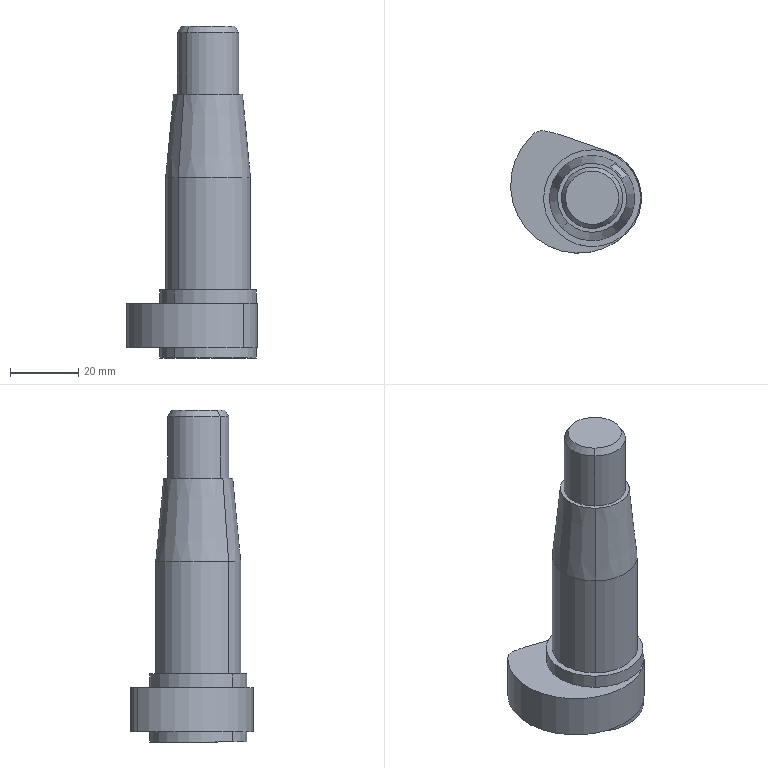Part | SolidWorks | features BaseBody 1 | 1 solid | 41 faces | box 38.423 x 35.937 x 97.5 mm | volume 48159 mm3 | plane 20 | cylinder 17 | cone 4 | commonest cylinder face diameters 28.5 x4 18 x2 25 x2 29 x2 6 x1 9 x1
STEP:
#1=CARTESIAN_POINT('',(-35.401,-41.494,71.636));
#2=VERTEX_POINT('',#1);
#3=CARTESIAN_POINT('',(-35.401,-41.494,85.05));
#4=VERTEX_POINT('',#3);
#5=CARTESIAN_POINT('',(-35.401,-41.494,99.25));
#6=DIRECTION('',(0.,0.,1.));
#7=VECTOR('',#6,1000.);
#8=LINE('',#5,#7);
#9=EDGE_CURVE('',#2,#4,#8,.T.);
#10=ORIENTED_EDGE('',*,*,#9,.F.);
#11=CARTESIAN_POINT('',(-32.752,-45.734,71.636));
#12=VERTEX_POINT('',#11);
#13=CARTESIAN_POINT('',(-44.463,-50.104,71.636));
#14=DIRECTION('',(0.,0.,-1.));
#15=DIRECTION('',(0.7009,0.7133,0.));
#16=AXIS2_PLACEMENT_3D('',#13,#14,#15);
#17=CIRCLE('',#16,12.5);
#18=EDGE_CURVE('',#2,#12,#17,.T.);
#19=ORIENTED_EDGE('',*,*,#18,.T.);
#20=CARTESIAN_POINT('',(-32.752,-45.734,85.05));
#21=VERTEX_POINT('',#20);
#22=CARTESIAN_POINT('',(-32.752,-45.734,99.25));
#23=DIRECTION('',(0.,0.,1.));
#24=VECTOR('',#23,1000.);
#25=LINE('',#22,#24);
#26=EDGE_CURVE('',#12,#21,#25,.T.);
#27=ORIENTED_EDGE('',*,*,#26,.T.);
#28=CARTESIAN_POINT('',(-44.463,-50.104,85.05));
#29=DIRECTION('',(0.,0.,1.));
#30=DIRECTION('',(-0.7009,-0.7133,0.));
#31=AXIS2_PLACEMENT_3D('',#28,#29,#30);
#32=CIRCLE('',#31,12.5);
#33=EDGE_CURVE('',#21,#4,#32,.T.);
#34=ORIENTED_EDGE('',*,*,#33,.T.);
#35=EDGE_LOOP('',(#10,#19,#27,#34));
#36=FACE_BOUND('',#35,.T.);
#37=CARTESIAN_POINT('',(-53.224,-59.019,99.25));
#38=VERTEX_POINT('',#37);
#39=CARTESIAN_POINT('',(-35.702,-41.188,99.25));
#40=VERTEX_POINT('',#39);
#41=CARTESIAN_POINT('',(-44.463,-50.104,99.25));
#42=DIRECTION('',(0.,0.,1.));
#43=DIRECTION('',(-0.7009,-0.7133,0.));
#44=AXIS2_PLACEMENT_3D('',#41,#42,#43);
#45=CIRCLE('',#44,12.5);
#46=EDGE_CURVE('',#38,#40,#45,.T.);
#47=ORIENTED_EDGE('',*,*,#46,.F.);
#48=CARTESIAN_POINT('',(-53.224,-59.019,66.25));
#49=VERTEX_POINT('',#48);
#50=CARTESIAN_POINT('',(-53.224,-59.019,99.25));
#51=DIRECTION('',(0.,0.,-1.));
#52=VECTOR('',#51,1000.);
#53=LINE('',#50,#52);
#54=EDGE_CURVE('',#38,#49,#53,.T.);
#55=ORIENTED_EDGE('',*,*,#54,.T.);
#56=CARTESIAN_POINT('',(-35.702,-41.188,66.25));
#57=VERTEX_POINT('',#56);
#58=CARTESIAN_POINT('',(-44.463,-50.104,66.25));
#59=DIRECTION('',(0.,0.,-1.));
#60=DIRECTION('',(0.7009,0.7133,0.));
#61=AXIS2_PLACEMENT_3D('',#58,#59,#60);
#62=CIRCLE('',#61,12.5);
#63=EDGE_CURVE('',#57,#49,#62,.T.);
#64=ORIENTED_EDGE('',*,*,#63,.F.);
#65=CARTESIAN_POINT('',(-35.702,-41.188,99.25));
#66=DIRECTION('',(0.,0.,-1.));
#67=VECTOR('',#66,1000.);
#68=LINE('',#65,#67);
#69=EDGE_CURVE('',#40,#57,#68,.T.);
#70=ORIENTED_EDGE('',*,*,#69,.F.);
#71=EDGE_LOOP('',(#47,#55,#64,#70));
#72=FACE_OUTER_BOUND('',#71,.T.);
#73=CARTESIAN_POINT('',(-44.463,-50.104,99.25));
#74=DIRECTION('',(0.,0.,-1.));
#75=DIRECTION('',(0.7009,0.7133,0.));
#76=AXIS2_PLACEMENT_3D('',#73,#74,#75);
#77=CYLINDRICAL_SURFACE('',#76,12.5);
#78=ADVANCED_FACE('',(#36,#72),#77,.T.);
#79=CARTESIAN_POINT('',(-34.3,-39.762,62.25));
#80=VERTEX_POINT('',#79);
#81=CARTESIAN_POINT('',(-39.674,-36.417,62.25));
#82=VERTEX_POINT('',#81);
#83=CARTESIAN_POINT('',(-44.463,-50.104,62.25));
#84=DIRECTION('',(0.,0.,1.));
#85=DIRECTION('',(-0.7009,-0.7133,0.));
#86=AXIS2_PLACEMENT_3D('',#83,#84,#85);
#87=CIRCLE('',#86,14.5);
#88=EDGE_CURVE('',#80,#82,#87,.T.);
#89=ORIENTED_EDGE('',*,*,#88,.F.);
#90=CARTESIAN_POINT('',(-34.3,-39.762,49.25));
#91=VERTEX_POINT('',#90);
#92=CARTESIAN_POINT('',(-34.3,-39.762,62.25));
#93=DIRECTION('',(0.,0.,-1.));
#94=VECTOR('',#93,1000.);
#95=LINE('',#92,#94);
#96=EDGE_CURVE('',#80,#91,#95,.T.);
#97=ORIENTED_EDGE('',*,*,#96,.T.);
#98=CARTESIAN_POINT('',(-39.674,-36.417,49.25));
#99=VERTEX_POINT('',#98);
#100=CARTESIAN_POINT('',(-44.463,-50.104,49.25));
#101=DIRECTION('',(0.,0.,1.));
#102=DIRECTION('',(-0.7009,-0.7133,0.));
#103=AXIS2_PLACEMENT_3D('',#100,#101,#102);
#104=CIRCLE('',#103,14.5);
#105=EDGE_CURVE('',#91,#99,#104,.T.);
#106=ORIENTED_EDGE('',*,*,#105,.T.);
#107=CARTESIAN_POINT('',(-39.674,-36.417,62.25));
#108=DIRECTION('',(0.,0.,-1.));
#109=VECTOR('',#108,1000.);
#110=LINE('',#107,#109);
#111=EDGE_CURVE('',#82,#99,#110,.T.);
#112=ORIENTED_EDGE('',*,*,#111,.F.);
#113=EDGE_LOOP('',(#89,#97,#106,#112));
#114=FACE_OUTER_BOUND('',#113,.T.);
#115=CARTESIAN_POINT('',(-44.463,-50.104,62.25));
#116=DIRECTION('',(0.,0.,-1.));
#117=DIRECTION('',(0.7009,0.7133,0.));
#118=AXIS2_PLACEMENT_3D('',#115,#116,#117);
#119=CYLINDRICAL_SURFACE('',#118,14.5);
#120=ADVANCED_FACE('',(#114),#119,.T.);
#121=CARTESIAN_POINT('',(-54.451,-60.268,46.25));
#122=VERTEX_POINT('',#121);
#123=CARTESIAN_POINT('',(-36.413,-38.345,46.25));
#124=VERTEX_POINT('',#123);
#125=CARTESIAN_POINT('',(-44.463,-50.104,46.25));
#126=DIRECTION('',(0.,0.,-1.));
#127=DIRECTION('',(0.7009,0.7133,0.));
#128=AXIS2_PLACEMENT_3D('',#125,#126,#127);
#129=CIRCLE('',#128,14.25);
#130=EDGE_CURVE('',#122,#124,#129,.T.);
#131=ORIENTED_EDGE('',*,*,#130,.F.);
#132=CARTESIAN_POINT('',(-54.451,-60.268,49.25));
#133=VERTEX_POINT('',#132);
#134=CARTESIAN_POINT('',(-54.451,-60.268,46.25));
#135=DIRECTION('',(0.,0.,1.));
#136=VECTOR('',#135,1000.);
#137=LINE('',#134,#136);
#138=EDGE_CURVE('',#122,#133,#137,.T.);
#139=ORIENTED_EDGE('',*,*,#138,.T.);
#140=CARTESIAN_POINT('',(-36.413,-38.345,49.25));
#141=VERTEX_POINT('',#140);
#142=CARTESIAN_POINT('',(-44.463,-50.104,49.25));
#143=DIRECTION('',(0.,0.,1.));
#144=DIRECTION('',(-0.7009,-0.7133,0.));
#145=AXIS2_PLACEMENT_3D('',#142,#143,#144);
#146=CIRCLE('',#145,14.25);
#147=EDGE_CURVE('',#141,#133,#146,.T.);
#148=ORIENTED_EDGE('',*,*,#147,.F.);
#149=CARTESIAN_POINT('',(-36.413,-38.345,46.25));
#150=DIRECTION('',(0.,0.,1.));
#151=VECTOR('',#150,1000.);
#152=LINE('',#149,#151);
#153=EDGE_CURVE('',#124,#141,#152,.T.);
#154=ORIENTED_EDGE('',*,*,#153,.F.);
#155=EDGE_LOOP('',(#131,#139,#148,#154));
#156=FACE_OUTER_BOUND('',#155,.T.);
#157=CARTESIAN_POINT('',(-44.463,-50.104,46.25));
#158=DIRECTION('',(0.,0.,1.));
#159=DIRECTION('',(-0.7009,-0.7133,0.));
#160=AXIS2_PLACEMENT_3D('',#157,#158,#159);
#161=CYLINDRICAL_SURFACE('',#160,14.25);
#162=ADVANCED_FACE('',(#156),#161,.T.);
#163=CARTESIAN_POINT('',(-51.571,-57.337,123.75));
#164=VERTEX_POINT('',#163);
#165=CARTESIAN_POINT('',(-37.355,-42.871,123.75));
#166=VERTEX_POINT('',#165);
#167=CARTESIAN_POINT('',(-44.463,-50.104,123.75));
#168=DIRECTION('',(0.,0.,-1.));
#169=DIRECTION('',(0.7009,0.7133,0.));
#170=AXIS2_PLACEMENT_3D('',#167,#168,#169);
#171=CIRCLE('',#170,10.141);
#172=EDGE_CURVE('',#164,#166,#171,.T.);
#173=ORIENTED_EDGE('',*,*,#172,.T.);
#174=CARTESIAN_POINT('',(-37.071,-42.582,119.547));
#175=VERTEX_POINT('',#174);
#176=CARTESIAN_POINT('',(-35.702,-41.188,99.25));
#177=DIRECTION('',(0.06718,0.06836,-0.9954));
#178=VECTOR('',#177,1000.);
#179=LINE('',#176,#178);
#180=EDGE_CURVE('',#166,#175,#179,.T.);
#181=ORIENTED_EDGE('',*,*,#180,.T.);
#182=CARTESIAN_POINT('',(-39.052,-41.03,119.351));
#183=VERTEX_POINT('',#182);
#184=CARTESIAN_POINT('',(-37.071,-42.582,119.547));
#185=CARTESIAN_POINT('',(-37.371,-42.288,119.547));
#186=CARTESIAN_POINT('',(-37.69,-42.007,119.531));
#187=CARTESIAN_POINT('',(-38.352,-41.489,119.467));
#188=CARTESIAN_POINT('',(-38.696,-41.25,119.418));
#189=CARTESIAN_POINT('',(-39.052,-41.03,119.351));
#190=B_SPLINE_CURVE_WITH_KNOTS('',3,(#184,#185,#186,#187,#188,#189),.UNSPECIFIED.,.F.,.F.,(4,2,4),(0.002522,0.003775,0.005027),.UNSPECIFIED.);
#191=EDGE_CURVE('',#175,#183,#190,.T.);
#192=ORIENTED_EDGE('',*,*,#191,.T.);
#193=CARTESIAN_POINT('',(-37.921,-39.88,103.01));
#194=VERTEX_POINT('',#193);
#195=CARTESIAN_POINT('',(-37.921,-39.88,103.01));
#196=CARTESIAN_POINT('',(-37.971,-39.931,103.745));
#197=CARTESIAN_POINT('',(-38.022,-39.983,104.479));
#198=CARTESIAN_POINT('',(-38.398,-40.365,109.927));
#199=CARTESIAN_POINT('',(-38.724,-40.697,114.639));
#200=CARTESIAN_POINT('',(-39.052,-41.03,119.351));
#201=B_SPLINE_CURVE_WITH_KNOTS('',3,(#195,#196,#197,#198,#199,#200),.UNSPECIFIED.,.F.,.F.,(4,2,4),(0.,0.1349,1.),.UNSPECIFIED.);
#202=EDGE_CURVE('',#194,#183,#201,.T.);
#203=ORIENTED_EDGE('',*,*,#202,.F.);
#204=CARTESIAN_POINT('',(-35.947,-41.438,102.891));
#205=VERTEX_POINT('',#204);
#206=CARTESIAN_POINT('',(-37.921,-39.88,103.01));
#207=CARTESIAN_POINT('',(-37.204,-40.329,102.926));
#208=CARTESIAN_POINT('',(-36.546,-40.849,102.891));
#209=CARTESIAN_POINT('',(-35.947,-41.438,102.891));
#210=B_SPLINE_CURVE_WITH_KNOTS('',3,(#206,#207,#208,#209),.UNSPECIFIED.,.F.,.F.,(4,4),(0.,0.002514),.UNSPECIFIED.);
#211=EDGE_CURVE('',#194,#205,#210,.T.);
#212=ORIENTED_EDGE('',*,*,#211,.T.);
#213=CARTESIAN_POINT('',(-35.702,-41.188,99.25));
#214=DIRECTION('',(0.06718,0.06836,-0.9954));
#215=VECTOR('',#214,1000.);
#216=LINE('',#213,#215);
#217=EDGE_CURVE('',#205,#40,#216,.T.);
#218=ORIENTED_EDGE('',*,*,#217,.T.);
#219=CARTESIAN_POINT('',(-44.463,-50.104,99.25));
#220=DIRECTION('',(0.,0.,1.));
#221=DIRECTION('',(-0.7009,-0.7133,0.));
#222=AXIS2_PLACEMENT_3D('',#219,#220,#221);
#223=CIRCLE('',#222,12.5);
#224=EDGE_CURVE('',#40,#38,#223,.T.);
#225=ORIENTED_EDGE('',*,*,#224,.T.);
#226=CARTESIAN_POINT('',(-53.224,-59.019,99.25));
#227=DIRECTION('',(-0.06718,-0.06836,-0.9954));
#228=VECTOR('',#227,1000.);
#229=LINE('',#226,#228);
#230=EDGE_CURVE('',#164,#38,#229,.T.);
#231=ORIENTED_EDGE('',*,*,#230,.F.);
#232=EDGE_LOOP('',(#173,#181,#192,#203,#212,#218,#225,#231));
#233=FACE_OUTER_BOUND('',#232,.T.);
#234=CARTESIAN_POINT('',(-44.463,-50.104,99.25));
#235=DIRECTION('',(0.,0.,-1.));
#236=DIRECTION('',(-0.7009,-0.7133,0.));
#237=AXIS2_PLACEMENT_3D('',#234,#235,#236);
#238=CONICAL_SURFACE('',#237,12.5,0.09599);
#239=ADVANCED_FACE('',(#233),#238,.T.);
#240=CARTESIAN_POINT('',(-38.155,-43.685,141.75));
#241=VERTEX_POINT('',#240);
#242=CARTESIAN_POINT('',(-50.771,-56.523,141.75));
#243=VERTEX_POINT('',#242);
#244=CARTESIAN_POINT('',(-44.463,-50.104,141.75));
#245=DIRECTION('',(0.,0.,-1.));
#246=DIRECTION('',(0.7009,0.7133,0.));
#247=AXIS2_PLACEMENT_3D('',#244,#245,#246);
#248=CIRCLE('',#247,9.);
#249=EDGE_CURVE('',#241,#243,#248,.T.);
#250=ORIENTED_EDGE('',*,*,#249,.T.);
#251=CARTESIAN_POINT('',(-50.771,-56.523,123.75));
#252=VERTEX_POINT('',#251);
#253=CARTESIAN_POINT('',(-50.771,-56.523,169.206));
#254=DIRECTION('',(0.,0.,-1.));
#255=VECTOR('',#254,1000.);
#256=LINE('',#253,#255);
#257=EDGE_CURVE('',#243,#252,#256,.T.);
#258=ORIENTED_EDGE('',*,*,#257,.T.);
#259=CARTESIAN_POINT('',(-38.155,-43.685,123.75));
#260=VERTEX_POINT('',#259);
#261=CARTESIAN_POINT('',(-44.463,-50.104,123.75));
#262=DIRECTION('',(0.,0.,1.));
#263=DIRECTION('',(0.7009,0.7133,0.));
#264=AXIS2_PLACEMENT_3D('',#261,#262,#263);
#265=CIRCLE('',#264,9.);
#266=EDGE_CURVE('',#252,#260,#265,.T.);
#267=ORIENTED_EDGE('',*,*,#266,.T.);
#268=CARTESIAN_POINT('',(-38.155,-43.685,169.206));
#269=DIRECTION('',(0.,0.,-1.));
#270=VECTOR('',#269,1000.);
#271=LINE('',#268,#270);
#272=EDGE_CURVE('',#241,#260,#271,.T.);
#273=ORIENTED_EDGE('',*,*,#272,.F.);
#274=EDGE_LOOP('',(#250,#258,#267,#273));
#275=FACE_OUTER_BOUND('',#274,.T.);
#276=CARTESIAN_POINT('',(-44.463,-50.104,169.206));
#277=DIRECTION('',(0.,0.,-1.));
#278=DIRECTION('',(0.7009,0.7133,0.));
#279=AXIS2_PLACEMENT_3D('',#276,#277,#278);
#280=CYLINDRICAL_SURFACE('',#279,9.);
#281=ADVANCED_FACE('',(#275),#280,.T.);
#282=CARTESIAN_POINT('',(-54.451,-60.268,62.25));
#283=VERTEX_POINT('',#282);
#284=CARTESIAN_POINT('',(-34.475,-39.94,62.25));
#285=VERTEX_POINT('',#284);
#286=CARTESIAN_POINT('',(-44.463,-50.104,62.25));
#287=DIRECTION('',(0.,0.,1.));
#288=DIRECTION('',(-0.7009,-0.7133,0.));
#289=AXIS2_PLACEMENT_3D('',#286,#287,#288);
#290=CIRCLE('',#289,14.25);
#291=EDGE_CURVE('',#283,#285,#290,.T.);
#292=ORIENTED_EDGE('',*,*,#291,.T.);
#293=CARTESIAN_POINT('',(-34.475,-39.94,66.25));
#294=VERTEX_POINT('',#293);
#295=CARTESIAN_POINT('',(-34.475,-39.94,46.25));
#296=DIRECTION('',(0.,0.,1.));
#297=VECTOR('',#296,1000.);
#298=LINE('',#295,#297);
#299=EDGE_CURVE('',#285,#294,#298,.T.);
#300=ORIENTED_EDGE('',*,*,#299,.T.);
#301=CARTESIAN_POINT('',(-54.451,-60.268,66.25));
#302=VERTEX_POINT('',#301);
#303=CARTESIAN_POINT('',(-44.463,-50.104,66.25));
#304=DIRECTION('',(0.,0.,-1.));
#305=DIRECTION('',(0.7009,0.7133,0.));
#306=AXIS2_PLACEMENT_3D('',#303,#304,#305);
#307=CIRCLE('',#306,14.25);
#308=EDGE_CURVE('',#294,#302,#307,.T.);
#309=ORIENTED_EDGE('',*,*,#308,.T.);
#310=CARTESIAN_POINT('',(-54.451,-60.268,46.25));
#311=DIRECTION('',(0.,0.,1.));
#312=VECTOR('',#311,1000.);
#313=LINE('',#310,#312);
#314=EDGE_CURVE('',#283,#302,#313,.T.);
#315=ORIENTED_EDGE('',*,*,#314,.F.);
#316=EDGE_LOOP('',(#292,#300,#309,#315));
#317=FACE_OUTER_BOUND('',#316,.T.);
#318=CARTESIAN_POINT('',(-44.463,-50.104,46.25));
#319=DIRECTION('',(0.,0.,1.));
#320=DIRECTION('',(-0.7009,-0.7133,0.));
#321=AXIS2_PLACEMENT_3D('',#318,#319,#320);
#322=CYLINDRICAL_SURFACE('',#321,14.25);
#323=ADVANCED_FACE('',(#317),#322,.T.);
#324=CARTESIAN_POINT('',(-49.962,-55.699,143.75));
#325=VERTEX_POINT('',#324);
#326=CARTESIAN_POINT('',(-38.964,-44.508,143.75));
#327=VERTEX_POINT('',#326);
#328=CARTESIAN_POINT('',(-44.463,-50.104,143.75));
#329=DIRECTION('',(0.,0.,1.));
#330=DIRECTION('',(0.7009,0.7133,0.));
#331=AXIS2_PLACEMENT_3D('',#328,#329,#330);
#332=CIRCLE('',#331,7.845);
#333=EDGE_CURVE('',#325,#327,#332,.T.);
#334=ORIENTED_EDGE('',*,*,#333,.F.);
#335=CARTESIAN_POINT('',(-50.771,-56.523,141.75));
#336=DIRECTION('',(-0.3505,-0.3566,-0.866));
#337=VECTOR('',#336,1000.);
#338=LINE('',#335,#337);
#339=EDGE_CURVE('',#325,#243,#338,.T.);
#340=ORIENTED_EDGE('',*,*,#339,.T.);
#341=ORIENTED_EDGE('',*,*,#249,.F.);
#342=CARTESIAN_POINT('',(-38.155,-43.685,141.75));
#343=DIRECTION('',(0.3505,0.3566,-0.866));
#344=VECTOR('',#343,1000.);
#345=LINE('',#342,#344);
#346=EDGE_CURVE('',#327,#241,#345,.T.);
#347=ORIENTED_EDGE('',*,*,#346,.F.);
#348=EDGE_LOOP('',(#334,#340,#341,#347));
#349=FACE_OUTER_BOUND('',#348,.T.);
#350=CARTESIAN_POINT('',(-44.463,-50.104,141.75));
#351=DIRECTION('',(0.,0.,-1.));
#352=DIRECTION('',(0.7009,0.7133,0.));
#353=AXIS2_PLACEMENT_3D('',#350,#351,#352);
#354=CONICAL_SURFACE('',#353,9.,0.5236);
#355=ADVANCED_FACE('',(#349),#354,.T.);
#356=CARTESIAN_POINT('',(-38.181,-49.126,85.05));
#357=VERTEX_POINT('',#356);
#358=CARTESIAN_POINT('',(-38.181,-49.126,71.636));
#359=VERTEX_POINT('',#358);
#360=CARTESIAN_POINT('',(-38.181,-49.126,85.05));
#361=DIRECTION('',(0.,0.,-1.));
#362=VECTOR('',#361,1000.);
#363=LINE('',#360,#362);
#364=EDGE_CURVE('',#357,#359,#363,.T.);
#365=ORIENTED_EDGE('',*,*,#364,.T.);
#366=CARTESIAN_POINT('',(-40.83,-44.886,71.636));
#367=VERTEX_POINT('',#366);
#368=CARTESIAN_POINT('',(-40.83,-44.886,71.636));
#369=DIRECTION('',(0.5299,-0.848,0.));
#370=VECTOR('',#369,1000.);
#371=LINE('',#368,#370);
#372=EDGE_CURVE('',#367,#359,#371,.T.);
#373=ORIENTED_EDGE('',*,*,#372,.F.);
#374=CARTESIAN_POINT('',(-40.83,-44.886,85.05));
#375=VERTEX_POINT('',#374);
#376=CARTESIAN_POINT('',(-40.83,-44.886,85.05));
#377=DIRECTION('',(0.,0.,-1.));
#378=VECTOR('',#377,1000.);
#379=LINE('',#376,#378);
#380=EDGE_CURVE('',#375,#367,#379,.T.);
#381=ORIENTED_EDGE('',*,*,#380,.F.);
#382=CARTESIAN_POINT('',(-40.83,-44.886,85.05));
#383=DIRECTION('',(0.5299,-0.848,0.));
#384=VECTOR('',#383,1000.);
#385=LINE('',#382,#384);
#386=EDGE_CURVE('',#375,#357,#385,.T.);
#387=ORIENTED_EDGE('',*,*,#386,.T.);
#388=EDGE_LOOP('',(#365,#373,#381,#387));
#389=FACE_OUTER_BOUND('',#388,.T.);
#390=CARTESIAN_POINT('',(-40.83,-44.886,85.05));
#391=DIRECTION('',(-0.848,-0.5299,0.));
#392=DIRECTION('',(-0.5299,0.848,0.));
#393=AXIS2_PLACEMENT_3D('',#390,#391,#392);
#394=PLANE('',#393);
#395=ADVANCED_FACE('',(#389),#394,.F.);
#396=CARTESIAN_POINT('',(-38.181,-49.126,71.636));
#397=DIRECTION('',(0.848,0.5299,0.));
#398=VECTOR('',#397,1000.);
#399=LINE('',#396,#398);
#400=EDGE_CURVE('',#359,#12,#399,.T.);
#401=ORIENTED_EDGE('',*,*,#400,.F.);
#402=ORIENTED_EDGE('',*,*,#364,.F.);
#403=CARTESIAN_POINT('',(-38.181,-49.126,85.05));
#404=DIRECTION('',(-0.848,-0.5299,0.));
#405=VECTOR('',#404,1000.);
#406=LINE('',#403,#405);
#407=EDGE_CURVE('',#21,#357,#406,.T.);
#408=ORIENTED_EDGE('',*,*,#407,.F.);
#409=ORIENTED_EDGE('',*,*,#26,.F.);
#410=EDGE_LOOP('',(#401,#402,#408,#409));
#411=FACE_OUTER_BOUND('',#410,.T.);
#412=CARTESIAN_POINT('',(-38.181,-49.126,71.636));
#413=DIRECTION('',(0.5299,-0.848,0.));
#414=DIRECTION('',(0.,0.,-1.));
#415=AXIS2_PLACEMENT_3D('',#412,#413,#414);
#416=PLANE('',#415);
#417=ADVANCED_FACE('',(#411),#416,.F.);
#418=ORIENTED_EDGE('',*,*,#9,.T.);
#419=CARTESIAN_POINT('',(-40.83,-44.886,85.05));
#420=DIRECTION('',(-0.848,-0.5299,0.));
#421=VECTOR('',#420,1000.);
#422=LINE('',#419,#421);
#423=EDGE_CURVE('',#4,#375,#422,.T.);
#424=ORIENTED_EDGE('',*,*,#423,.T.);
#425=ORIENTED_EDGE('',*,*,#380,.T.);
#426=CARTESIAN_POINT('',(-40.83,-44.886,71.636));
#427=DIRECTION('',(0.848,0.5299,0.));
#428=VECTOR('',#427,1000.);
#429=LINE('',#426,#428);
#430=EDGE_CURVE('',#367,#2,#429,.T.);
#431=ORIENTED_EDGE('',*,*,#430,.T.);
#432=EDGE_LOOP('',(#418,#424,#425,#431));
#433=FACE_OUTER_BOUND('',#432,.T.);
#434=CARTESIAN_POINT('',(-40.83,-44.886,71.636));
#435=DIRECTION('',(0.5299,-0.848,0.));
#436=DIRECTION('',(0.,0.,-1.));
#437=AXIS2_PLACEMENT_3D('',#434,#435,#436);
#438=PLANE('',#437);
#439=ADVANCED_FACE('',(#433),#438,.T.);
#440=ORIENTED_EDGE('',*,*,#430,.F.);
#441=ORIENTED_EDGE('',*,*,#372,.T.);
#442=ORIENTED_EDGE('',*,*,#400,.T.);
#443=ORIENTED_EDGE('',*,*,#18,.F.);
#444=EDGE_LOOP('',(#440,#441,#442,#443));
#445=FACE_OUTER_BOUND('',#444,.T.);
#446=CARTESIAN_POINT('',(-40.83,-44.886,71.636));
#447=DIRECTION('',(0.,0.,-1.));
#448=DIRECTION('',(0.,-1.,0.));
#449=AXIS2_PLACEMENT_3D('',#446,#447,#448);
#450=PLANE('',#449);
#451=ADVANCED_FACE('',(#445),#450,.F.);
#452=ORIENTED_EDGE('',*,*,#407,.T.);
#453=ORIENTED_EDGE('',*,*,#386,.F.);
#454=ORIENTED_EDGE('',*,*,#423,.F.);
#455=ORIENTED_EDGE('',*,*,#33,.F.);
#456=EDGE_LOOP('',(#452,#453,#454,#455));
#457=FACE_OUTER_BOUND('',#456,.T.);
#458=CARTESIAN_POINT('',(-40.83,-44.886,85.05));
#459=DIRECTION('',(0.,0.,1.));
#460=DIRECTION('',(0.,-1.,0.));
#461=AXIS2_PLACEMENT_3D('',#458,#459,#460);
#462=PLANE('',#461);
#463=ADVANCED_FACE('',(#457),#462,.F.);
#464=CARTESIAN_POINT('',(-31.241,-44.79,46.25));
#465=VERTEX_POINT('',#464);
#466=CARTESIAN_POINT('',(-35.995,-47.76,46.25));
#467=VERTEX_POINT('',#466);
#468=CARTESIAN_POINT('',(-43.138,-52.224,46.25));
#469=DIRECTION('',(-0.848,-0.5299,0.));
#470=VECTOR('',#469,1000.);
#471=LINE('',#468,#470);
#472=EDGE_CURVE('',#465,#467,#471,.T.);
#473=ORIENTED_EDGE('',*,*,#472,.T.);
#474=CARTESIAN_POINT('',(-35.995,-47.76,53.733));
#475=VERTEX_POINT('',#474);
#476=CARTESIAN_POINT('',(-35.995,-47.76,53.733));
#477=DIRECTION('',(0.,0.,-1.));
#478=VECTOR('',#477,1000.);
#479=LINE('',#476,#478);
#480=EDGE_CURVE('',#475,#467,#479,.T.);
#481=ORIENTED_EDGE('',*,*,#480,.F.);
#482=CARTESIAN_POINT('',(-31.026,-44.655,53.733));
#483=VERTEX_POINT('',#482);
#484=CARTESIAN_POINT('',(-35.995,-47.76,53.733));
#485=DIRECTION('',(-0.848,-0.5299,0.));
#486=VECTOR('',#485,1000.);
#487=LINE('',#484,#486);
#488=EDGE_CURVE('',#483,#475,#487,.T.);
#489=ORIENTED_EDGE('',*,*,#488,.F.);
#490=CARTESIAN_POINT('',(-31.026,-44.655,49.25));
#491=VERTEX_POINT('',#490);
#492=CARTESIAN_POINT('',(-31.026,-44.655,62.25));
#493=DIRECTION('',(0.,0.,1.));
#494=VECTOR('',#493,1000.);
#495=LINE('',#492,#494);
#496=EDGE_CURVE('',#491,#483,#495,.T.);
#497=ORIENTED_EDGE('',*,*,#496,.F.);
#498=CARTESIAN_POINT('',(-31.241,-44.79,49.25));
#499=VERTEX_POINT('',#498);
#500=CARTESIAN_POINT('',(-43.138,-52.224,49.25));
#501=DIRECTION('',(0.848,0.5299,0.));
#502=VECTOR('',#501,1000.);
#503=LINE('',#500,#502);
#504=EDGE_CURVE('',#499,#491,#503,.T.);
#505=ORIENTED_EDGE('',*,*,#504,.F.);
#506=CARTESIAN_POINT('',(-31.241,-44.79,46.25));
#507=DIRECTION('',(0.,0.,1.));
#508=VECTOR('',#507,1000.);
#509=LINE('',#506,#508);
#510=EDGE_CURVE('',#465,#499,#509,.T.);
#511=ORIENTED_EDGE('',*,*,#510,.F.);
#512=EDGE_LOOP('',(#473,#481,#489,#497,#505,#511));
#513=FACE_OUTER_BOUND('',#512,.T.);
#514=CARTESIAN_POINT('',(-35.995,-47.76,40.466));
#515=DIRECTION('',(0.5299,-0.848,0.));
#516=DIRECTION('',(0.,0.,-1.));
#517=AXIS2_PLACEMENT_3D('',#514,#515,#516);
#518=PLANE('',#517);
#519=ADVANCED_FACE('',(#513),#518,.F.);
#520=CARTESIAN_POINT('',(-38.644,-43.52,46.25));
#521=VERTEX_POINT('',#520);
#522=CARTESIAN_POINT('',(-37.32,-45.64,46.25));
#523=DIRECTION('',(-0.5299,0.848,0.));
#524=VECTOR('',#523,1000.);
#525=LINE('',#522,#524);
#526=EDGE_CURVE('',#467,#521,#525,.T.);
#527=ORIENTED_EDGE('',*,*,#526,.T.);
#528=CARTESIAN_POINT('',(-38.644,-43.52,53.733));
#529=VERTEX_POINT('',#528);
#530=CARTESIAN_POINT('',(-38.644,-43.52,53.733));
#531=DIRECTION('',(0.,0.,-1.));
#532=VECTOR('',#531,1000.);
#533=LINE('',#530,#532);
#534=EDGE_CURVE('',#529,#521,#533,.T.);
#535=ORIENTED_EDGE('',*,*,#534,.F.);
#536=CARTESIAN_POINT('',(-38.644,-43.52,53.733));
#537=DIRECTION('',(0.5299,-0.848,0.));
#538=VECTOR('',#537,1000.);
#539=LINE('',#536,#538);
#540=EDGE_CURVE('',#529,#475,#539,.T.);
#541=ORIENTED_EDGE('',*,*,#540,.T.);
#542=ORIENTED_EDGE('',*,*,#480,.T.);
#543=EDGE_LOOP('',(#527,#535,#541,#542));
#544=FACE_OUTER_BOUND('',#543,.T.);
#545=CARTESIAN_POINT('',(-38.644,-43.52,53.733));
#546=DIRECTION('',(-0.848,-0.5299,0.));
#547=DIRECTION('',(-0.5299,0.848,0.));
#548=AXIS2_PLACEMENT_3D('',#545,#546,#547);
#549=PLANE('',#548);
#550=ADVANCED_FACE('',(#544),#549,.F.);
#551=CARTESIAN_POINT('',(-33.675,-40.415,49.25));
#552=VERTEX_POINT('',#551);
#553=CARTESIAN_POINT('',(-33.675,-40.415,53.733));
#554=VERTEX_POINT('',#553);
#555=CARTESIAN_POINT('',(-33.675,-40.415,62.25));
#556=DIRECTION('',(0.,0.,1.));
#557=VECTOR('',#556,1000.);
#558=LINE('',#555,#557);
#559=EDGE_CURVE('',#552,#554,#558,.T.);
#560=ORIENTED_EDGE('',*,*,#559,.T.);
#561=CARTESIAN_POINT('',(-38.644,-43.52,53.733));
#562=DIRECTION('',(-0.848,-0.5299,0.));
#563=VECTOR('',#562,1000.);
#564=LINE('',#561,#563);
#565=EDGE_CURVE('',#554,#529,#564,.T.);
#566=ORIENTED_EDGE('',*,*,#565,.T.);
#567=ORIENTED_EDGE('',*,*,#534,.T.);
#568=CARTESIAN_POINT('',(-38.258,-43.279,46.25));
#569=VERTEX_POINT('',#568);
#570=CARTESIAN_POINT('',(-45.788,-47.984,46.25));
#571=DIRECTION('',(-0.848,-0.5299,0.));
#572=VECTOR('',#571,1000.);
#573=LINE('',#570,#572);
#574=EDGE_CURVE('',#569,#521,#573,.T.);
#575=ORIENTED_EDGE('',*,*,#574,.F.);
#576=CARTESIAN_POINT('',(-38.258,-43.279,49.25));
#577=VERTEX_POINT('',#576);
#578=CARTESIAN_POINT('',(-38.258,-43.279,43.06));
#579=DIRECTION('',(0.,0.,1.));
#580=VECTOR('',#579,1000.);
#581=LINE('',#578,#580);
#582=EDGE_CURVE('',#569,#577,#581,.T.);
#583=ORIENTED_EDGE('',*,*,#582,.T.);
#584=CARTESIAN_POINT('',(-45.788,-47.984,49.25));
#585=DIRECTION('',(0.848,0.5299,0.));
#586=VECTOR('',#585,1000.);
#587=LINE('',#584,#586);
#588=EDGE_CURVE('',#577,#552,#587,.T.);
#589=ORIENTED_EDGE('',*,*,#588,.T.);
#590=EDGE_LOOP('',(#560,#566,#567,#575,#583,#589));
#591=FACE_OUTER_BOUND('',#590,.T.);
#592=CARTESIAN_POINT('',(-38.644,-43.52,40.466));
#593=DIRECTION('',(0.5299,-0.848,0.));
#594=DIRECTION('',(0.,0.,-1.));
#595=AXIS2_PLACEMENT_3D('',#592,#593,#594);
#596=PLANE('',#595);
#597=ADVANCED_FACE('',(#591),#596,.T.);
#598=ORIENTED_EDGE('',*,*,#488,.T.);
#599=ORIENTED_EDGE('',*,*,#540,.F.);
#600=ORIENTED_EDGE('',*,*,#565,.F.);
#601=CARTESIAN_POINT('',(-44.463,-50.104,53.733));
#602=DIRECTION('',(0.,0.,1.));
#603=DIRECTION('',(-0.7009,-0.7133,0.));
#604=AXIS2_PLACEMENT_3D('',#601,#602,#603);
#605=CIRCLE('',#604,14.5);
#606=EDGE_CURVE('',#483,#554,#605,.T.);
#607=ORIENTED_EDGE('',*,*,#606,.F.);
#608=EDGE_LOOP('',(#598,#599,#600,#607));
#609=FACE_OUTER_BOUND('',#608,.T.);
#610=CARTESIAN_POINT('',(-38.644,-43.52,53.733));
#611=DIRECTION('',(0.,0.,1.));
#612=DIRECTION('',(0.,-1.,0.));
#613=AXIS2_PLACEMENT_3D('',#610,#611,#612);
#614=PLANE('',#613);
#615=ADVANCED_FACE('',(#609),#614,.F.);
#616=ORIENTED_EDGE('',*,*,#153,.T.);
#617=CARTESIAN_POINT('',(-39.786,-41.778,49.25));
#618=VERTEX_POINT('',#617);
#619=CARTESIAN_POINT('',(-30.821,-32.655,49.25));
#620=DIRECTION('',(-0.7009,-0.7133,0.));
#621=VECTOR('',#620,1000.);
#622=LINE('',#619,#621);
#623=EDGE_CURVE('',#141,#618,#622,.T.);
#624=ORIENTED_EDGE('',*,*,#623,.T.);
#625=CARTESIAN_POINT('',(-39.786,-41.778,46.25));
#626=VERTEX_POINT('',#625);
#627=CARTESIAN_POINT('',(-39.786,-41.778,43.06));
#628=DIRECTION('',(0.,0.,-1.));
#629=VECTOR('',#628,1000.);
#630=LINE('',#627,#629);
#631=EDGE_CURVE('',#618,#626,#630,.T.);
#632=ORIENTED_EDGE('',*,*,#631,.T.);
#633=CARTESIAN_POINT('',(-46.246,-48.352,46.25));
#634=DIRECTION('',(-0.7009,-0.7133,0.));
#635=VECTOR('',#634,1000.);
#636=LINE('',#633,#635);
#637=EDGE_CURVE('',#124,#626,#636,.T.);
#638=ORIENTED_EDGE('',*,*,#637,.F.);
#639=EDGE_LOOP('',(#616,#624,#632,#638));
#640=FACE_OUTER_BOUND('',#639,.T.);
#641=CARTESIAN_POINT('',(-30.821,-32.655,49.25));
#642=DIRECTION('',(0.7133,-0.7009,0.));
#643=DIRECTION('',(0.,0.,-1.));
#644=AXIS2_PLACEMENT_3D('',#641,#642,#643);
#645=PLANE('',#644);
#646=ADVANCED_FACE('',(#640),#645,.T.);
#647=CARTESIAN_POINT('',(-35.485,-44.535,119.351));
#648=VERTEX_POINT('',#647);
#649=CARTESIAN_POINT('',(-34.355,-43.384,103.01));
#650=VERTEX_POINT('',#649);
#651=CARTESIAN_POINT('',(-31.587,-40.568,111.65));
#652=DIRECTION('',(0.7133,-0.7009,0.));
#653=DIRECTION('',(0.,0.,1.));
#654=AXIS2_PLACEMENT_3D('',#651,#652,#653);
#655=CIRCLE('',#654,9.5);
#656=EDGE_CURVE('',#648,#650,#655,.T.);
#657=ORIENTED_EDGE('',*,*,#656,.F.);
#658=CARTESIAN_POINT('',(-34.355,-43.384,103.01));
#659=CARTESIAN_POINT('',(-34.405,-43.436,103.745));
#660=CARTESIAN_POINT('',(-34.456,-43.487,104.479));
#661=CARTESIAN_POINT('',(-34.832,-43.87,109.927));
#662=CARTESIAN_POINT('',(-35.158,-44.202,114.639));
#663=CARTESIAN_POINT('',(-35.485,-44.535,119.351));
#664=B_SPLINE_CURVE_WITH_KNOTS('',3,(#658,#659,#660,#661,#662,#663),.UNSPECIFIED.,.F.,.F.,(4,2,4),(0.,0.1349,1.),.UNSPECIFIED.);
#665=EDGE_CURVE('',#650,#648,#664,.T.);
#666=ORIENTED_EDGE('',*,*,#665,.F.);
#667=EDGE_LOOP('',(#657,#666));
#668=FACE_OUTER_BOUND('',#667,.T.);
#669=CARTESIAN_POINT('',(-31.587,-40.568,111.65));
#670=DIRECTION('',(0.7133,-0.7009,0.));
#671=DIRECTION('',(0.,0.,-1.));
#672=AXIS2_PLACEMENT_3D('',#669,#670,#671);
#673=PLANE('',#672);
#674=ADVANCED_FACE('',(#668),#673,.F.);
#675=ORIENTED_EDGE('',*,*,#202,.T.);
#676=CARTESIAN_POINT('',(-35.153,-37.063,111.65));
#677=DIRECTION('',(0.7133,-0.7009,0.));
#678=DIRECTION('',(0.,0.,1.));
#679=AXIS2_PLACEMENT_3D('',#676,#677,#678);
#680=CIRCLE('',#679,9.5);
#681=EDGE_CURVE('',#183,#194,#680,.T.);
#682=ORIENTED_EDGE('',*,*,#681,.T.);
#683=EDGE_LOOP('',(#675,#682));
#684=FACE_OUTER_BOUND('',#683,.T.);
#685=CARTESIAN_POINT('',(-35.153,-37.063,111.65));
#686=DIRECTION('',(0.7133,-0.7009,0.));
#687=DIRECTION('',(0.,0.,-1.));
#688=AXIS2_PLACEMENT_3D('',#685,#686,#687);
#689=PLANE('',#688);
#690=ADVANCED_FACE('',(#684),#689,.T.);
#691=ORIENTED_EDGE('',*,*,#656,.T.);
#692=CARTESIAN_POINT('',(-35.947,-41.438,102.891));
#693=CARTESIAN_POINT('',(-35.65,-41.731,102.891));
#694=CARTESIAN_POINT('',(-35.366,-42.041,102.9));
#695=CARTESIAN_POINT('',(-34.832,-42.693,102.939));
#696=CARTESIAN_POINT('',(-34.584,-43.032,102.968));
#697=CARTESIAN_POINT('',(-34.355,-43.384,103.01));
#698=B_SPLINE_CURVE_WITH_KNOTS('',3,(#692,#693,#694,#695,#696,#697),.UNSPECIFIED.,.F.,.F.,(4,2,4),(0.002514,0.003763,0.005012),.UNSPECIFIED.);
#699=EDGE_CURVE('',#205,#650,#698,.T.);
#700=ORIENTED_EDGE('',*,*,#699,.F.);
#701=ORIENTED_EDGE('',*,*,#211,.F.);
#702=ORIENTED_EDGE('',*,*,#681,.F.);
#703=ORIENTED_EDGE('',*,*,#191,.F.);
#704=CARTESIAN_POINT('',(-35.485,-44.535,119.351));
#705=CARTESIAN_POINT('',(-35.94,-43.826,119.486));
#706=CARTESIAN_POINT('',(-36.468,-43.175,119.547));
#707=CARTESIAN_POINT('',(-37.071,-42.582,119.547));
#708=B_SPLINE_CURVE_WITH_KNOTS('',3,(#704,#705,#706,#707),.UNSPECIFIED.,.F.,.F.,(4,4),(0.,0.002522),.UNSPECIFIED.);
#709=EDGE_CURVE('',#648,#175,#708,.T.);
#710=ORIENTED_EDGE('',*,*,#709,.F.);
#711=EDGE_LOOP('',(#691,#700,#701,#702,#703,#710));
#712=FACE_OUTER_BOUND('',#711,.T.);
#713=CARTESIAN_POINT('',(-35.153,-37.063,111.65));
#714=DIRECTION('',(0.7133,-0.7009,0.));
#715=DIRECTION('',(0.,0.,1.));
#716=AXIS2_PLACEMENT_3D('',#713,#714,#715);
#717=CYLINDRICAL_SURFACE('',#716,9.5);
#718=ADVANCED_FACE('',(#712),#717,.F.);
#719=ORIENTED_EDGE('',*,*,#339,.F.);
#720=CARTESIAN_POINT('',(-44.463,-50.104,143.75));
#721=DIRECTION('',(0.,0.,1.));
#722=DIRECTION('',(0.7009,0.7133,0.));
#723=AXIS2_PLACEMENT_3D('',#720,#721,#722);
#724=CIRCLE('',#723,7.845);
#725=EDGE_CURVE('',#327,#325,#724,.T.);
#726=ORIENTED_EDGE('',*,*,#725,.F.);
#727=ORIENTED_EDGE('',*,*,#346,.T.);
#728=CARTESIAN_POINT('',(-44.463,-50.104,141.75));
#729=DIRECTION('',(0.,0.,-1.));
#730=DIRECTION('',(0.7009,0.7133,0.));
#731=AXIS2_PLACEMENT_3D('',#728,#729,#730);
#732=CIRCLE('',#731,9.);
#733=EDGE_CURVE('',#243,#241,#732,.T.);
#734=ORIENTED_EDGE('',*,*,#733,.F.);
#735=EDGE_LOOP('',(#719,#726,#727,#734));
#736=FACE_OUTER_BOUND('',#735,.T.);
#737=CARTESIAN_POINT('',(-44.463,-50.104,141.75));
#738=DIRECTION('',(0.,0.,-1.));
#739=DIRECTION('',(0.7009,0.7133,0.));
#740=AXIS2_PLACEMENT_3D('',#737,#738,#739);
#741=CONICAL_SURFACE('',#740,9.,0.5236);
#742=ADVANCED_FACE('',(#736),#741,.T.);
#743=CARTESIAN_POINT('',(-60.534,-30.569,49.25));
#744=VERTEX_POINT('',#743);
#745=CARTESIAN_POINT('',(-61.543,-31.17,49.25));
#746=VERTEX_POINT('',#745);
#747=CARTESIAN_POINT('',(-59.534,-33.397,49.25));
#748=DIRECTION('',(0.,0.,1.));
#749=DIRECTION('',(-0.7009,-0.7133,0.));
#750=AXIS2_PLACEMENT_3D('',#747,#748,#749);
#751=CIRCLE('',#750,3.);
#752=EDGE_CURVE('',#744,#746,#751,.T.);
#753=ORIENTED_EDGE('',*,*,#752,.T.);
#754=CARTESIAN_POINT('',(-61.543,-31.17,62.25));
#755=VERTEX_POINT('',#754);
#756=CARTESIAN_POINT('',(-61.543,-31.17,62.25));
#757=DIRECTION('',(0.,0.,-1.));
#758=VECTOR('',#757,1000.);
#759=LINE('',#756,#758);
#760=EDGE_CURVE('',#755,#746,#759,.T.);
#761=ORIENTED_EDGE('',*,*,#760,.F.);
#762=CARTESIAN_POINT('',(-60.534,-30.569,62.25));
#763=VERTEX_POINT('',#762);
#764=CARTESIAN_POINT('',(-59.534,-33.397,62.25));
#765=DIRECTION('',(0.,0.,1.));
#766=DIRECTION('',(-0.7009,-0.7133,0.));
#767=AXIS2_PLACEMENT_3D('',#764,#765,#766);
#768=CIRCLE('',#767,3.);
#769=EDGE_CURVE('',#763,#755,#768,.T.);
#770=ORIENTED_EDGE('',*,*,#769,.F.);
#771=CARTESIAN_POINT('',(-60.534,-30.569,62.25));
#772=DIRECTION('',(0.,0.,-1.));
#773=VECTOR('',#772,1000.);
#774=LINE('',#771,#773);
#775=EDGE_CURVE('',#763,#744,#774,.T.);
#776=ORIENTED_EDGE('',*,*,#775,.T.);
#777=EDGE_LOOP('',(#753,#761,#770,#776));
#778=FACE_OUTER_BOUND('',#777,.T.);
#779=CARTESIAN_POINT('',(-59.534,-33.397,62.25));
#780=DIRECTION('',(0.,0.,-1.));
#781=DIRECTION('',(0.7009,0.7133,0.));
#782=AXIS2_PLACEMENT_3D('',#779,#780,#781);
#783=CYLINDRICAL_SURFACE('',#782,3.);
#784=ADVANCED_FACE('',(#778),#783,.T.);
#785=CARTESIAN_POINT('',(-58.109,-30.407,49.25));
#786=VERTEX_POINT('',#785);
#787=CARTESIAN_POINT('',(-59.034,-34.811,49.25));
#788=DIRECTION('',(0.,0.,1.));
#789=DIRECTION('',(-0.7009,-0.7133,0.));
#790=AXIS2_PLACEMENT_3D('',#787,#788,#789);
#791=CIRCLE('',#790,4.5);
#792=EDGE_CURVE('',#786,#744,#791,.T.);
#793=ORIENTED_EDGE('',*,*,#792,.T.);
#794=ORIENTED_EDGE('',*,*,#775,.F.);
#795=CARTESIAN_POINT('',(-58.109,-30.407,62.25));
#796=VERTEX_POINT('',#795);
#797=CARTESIAN_POINT('',(-59.034,-34.811,62.25));
#798=DIRECTION('',(0.,0.,1.));
#799=DIRECTION('',(-0.7009,-0.7133,0.));
#800=AXIS2_PLACEMENT_3D('',#797,#798,#799);
#801=CIRCLE('',#800,4.5);
#802=EDGE_CURVE('',#796,#763,#801,.T.);
#803=ORIENTED_EDGE('',*,*,#802,.F.);
#804=CARTESIAN_POINT('',(-58.109,-30.407,62.25));
#805=DIRECTION('',(0.,0.,-1.));
#806=VECTOR('',#805,1000.);
#807=LINE('',#804,#806);
#808=EDGE_CURVE('',#796,#786,#807,.T.);
#809=ORIENTED_EDGE('',*,*,#808,.T.);
#810=EDGE_LOOP('',(#793,#794,#803,#809));
#811=FACE_OUTER_BOUND('',#810,.T.);
#812=CARTESIAN_POINT('',(-59.034,-34.811,62.25));
#813=DIRECTION('',(0.,0.,-1.));
#814=DIRECTION('',(0.7009,0.7133,0.));
#815=AXIS2_PLACEMENT_3D('',#812,#813,#814);
#816=CYLINDRICAL_SURFACE('',#815,4.5);
#817=ADVANCED_FACE('',(#811),#816,.T.);
#818=CARTESIAN_POINT('',(-57.741,-30.493,49.25));
#819=VERTEX_POINT('',#818);
#820=CARTESIAN_POINT('',(-59.063,-35.315,49.25));
#821=DIRECTION('',(0.,0.,1.));
#822=DIRECTION('',(-0.7009,-0.7133,0.));
#823=AXIS2_PLACEMENT_3D('',#820,#821,#822);
#824=CIRCLE('',#823,5.);
#825=EDGE_CURVE('',#819,#786,#824,.T.);
#826=ORIENTED_EDGE('',*,*,#825,.T.);
#827=ORIENTED_EDGE('',*,*,#808,.F.);
#828=CARTESIAN_POINT('',(-57.741,-30.493,62.25));
#829=VERTEX_POINT('',#828);
#830=CARTESIAN_POINT('',(-59.063,-35.315,62.25));
#831=DIRECTION('',(0.,0.,1.));
#832=DIRECTION('',(-0.7009,-0.7133,0.));
#833=AXIS2_PLACEMENT_3D('',#830,#831,#832);
#834=CIRCLE('',#833,5.);
#835=EDGE_CURVE('',#829,#796,#834,.T.);
#836=ORIENTED_EDGE('',*,*,#835,.F.);
#837=CARTESIAN_POINT('',(-57.741,-30.493,62.25));
#838=DIRECTION('',(0.,0.,-1.));
#839=VECTOR('',#838,1000.);
#840=LINE('',#837,#839);
#841=EDGE_CURVE('',#829,#819,#840,.T.);
#842=ORIENTED_EDGE('',*,*,#841,.T.);
#843=EDGE_LOOP('',(#826,#827,#836,#842));
#844=FACE_OUTER_BOUND('',#843,.T.);
#845=CARTESIAN_POINT('',(-59.063,-35.315,62.25));
#846=DIRECTION('',(0.,0.,-1.));
#847=DIRECTION('',(0.7009,0.7133,0.));
#848=AXIS2_PLACEMENT_3D('',#845,#846,#847);
#849=CYLINDRICAL_SURFACE('',#848,5.);
#850=ADVANCED_FACE('',(#844),#849,.T.);
#851=CARTESIAN_POINT('',(-53.772,-31.485,49.25));
#852=VERTEX_POINT('',#851);
#853=CARTESIAN_POINT('',(-61.137,-52.533,49.25));
#854=DIRECTION('',(0.,0.,1.));
#855=DIRECTION('',(-0.7009,-0.7133,0.));
#856=AXIS2_PLACEMENT_3D('',#853,#854,#855);
#857=CIRCLE('',#856,22.3);
#858=EDGE_CURVE('',#852,#819,#857,.T.);
#859=ORIENTED_EDGE('',*,*,#858,.T.);
#860=ORIENTED_EDGE('',*,*,#841,.F.);
#861=CARTESIAN_POINT('',(-53.772,-31.485,62.25));
#862=VERTEX_POINT('',#861);
#863=CARTESIAN_POINT('',(-61.137,-52.533,62.25));
#864=DIRECTION('',(0.,0.,1.));
#865=DIRECTION('',(-0.7009,-0.7133,0.));
#866=AXIS2_PLACEMENT_3D('',#863,#864,#865);
#867=CIRCLE('',#866,22.3);
#868=EDGE_CURVE('',#862,#829,#867,.T.);
#869=ORIENTED_EDGE('',*,*,#868,.F.);
#870=CARTESIAN_POINT('',(-53.772,-31.485,62.25));
#871=DIRECTION('',(0.,0.,-1.));
#872=VECTOR('',#871,1000.);
#873=LINE('',#870,#872);
#874=EDGE_CURVE('',#862,#852,#873,.T.);
#875=ORIENTED_EDGE('',*,*,#874,.T.);
#876=EDGE_LOOP('',(#859,#860,#869,#875));
#877=FACE_OUTER_BOUND('',#876,.T.);
#878=CARTESIAN_POINT('',(-61.137,-52.533,62.25));
#879=DIRECTION('',(0.,0.,-1.));
#880=DIRECTION('',(0.7009,0.7133,0.));
#881=AXIS2_PLACEMENT_3D('',#878,#879,#880);
#882=CYLINDRICAL_SURFACE('',#881,22.3);
#883=ADVANCED_FACE('',(#877),#882,.T.);
#884=CARTESIAN_POINT('',(-39.674,-36.417,49.25));
#885=DIRECTION('',(-0.9439,0.3303,0.));
#886=VECTOR('',#885,1000.);
#887=LINE('',#884,#886);
#888=EDGE_CURVE('',#99,#852,#887,.T.);
#889=ORIENTED_EDGE('',*,*,#888,.T.);
#890=ORIENTED_EDGE('',*,*,#874,.F.);
#891=CARTESIAN_POINT('',(-39.674,-36.417,62.25));
#892=DIRECTION('',(-0.9439,0.3303,0.));
#893=VECTOR('',#892,1000.);
#894=LINE('',#891,#893);
#895=EDGE_CURVE('',#82,#862,#894,.T.);
#896=ORIENTED_EDGE('',*,*,#895,.F.);
#897=ORIENTED_EDGE('',*,*,#111,.T.);
#898=EDGE_LOOP('',(#889,#890,#896,#897));
#899=FACE_OUTER_BOUND('',#898,.T.);
#900=CARTESIAN_POINT('',(-39.674,-36.417,62.25));
#901=DIRECTION('',(-0.3303,-0.9439,0.));
#902=DIRECTION('',(-0.9439,0.3303,0.));
#903=AXIS2_PLACEMENT_3D('',#900,#901,#902);
#904=PLANE('',#903);
#905=ADVANCED_FACE('',(#899),#904,.F.);
#906=CARTESIAN_POINT('',(-62.651,-32.231,49.25));
#907=VERTEX_POINT('',#906);
#908=CARTESIAN_POINT('',(-34.121,-60.267,49.25));
#909=VERTEX_POINT('',#908);
#910=CARTESIAN_POINT('',(-48.386,-46.249,49.25));
#911=DIRECTION('',(0.,0.,1.));
#912=DIRECTION('',(-0.7009,-0.7133,0.));
#913=AXIS2_PLACEMENT_3D('',#910,#911,#912);
#914=CIRCLE('',#913,20.);
#915=EDGE_CURVE('',#907,#909,#914,.T.);
#916=ORIENTED_EDGE('',*,*,#915,.T.);
#917=CARTESIAN_POINT('',(-34.121,-60.267,62.25));
#918=VERTEX_POINT('',#917);
#919=CARTESIAN_POINT('',(-34.121,-60.267,62.25));
#920=DIRECTION('',(0.,0.,-1.));
#921=VECTOR('',#920,1000.);
#922=LINE('',#919,#921);
#923=EDGE_CURVE('',#918,#909,#922,.T.);
#924=ORIENTED_EDGE('',*,*,#923,.F.);
#925=CARTESIAN_POINT('',(-62.651,-32.231,62.25));
#926=VERTEX_POINT('',#925);
#927=CARTESIAN_POINT('',(-48.386,-46.249,62.25));
#928=DIRECTION('',(0.,0.,1.));
#929=DIRECTION('',(-0.7009,-0.7133,0.));
#930=AXIS2_PLACEMENT_3D('',#927,#928,#929);
#931=CIRCLE('',#930,20.);
#932=EDGE_CURVE('',#926,#918,#931,.T.);
#933=ORIENTED_EDGE('',*,*,#932,.F.);
#934=CARTESIAN_POINT('',(-62.651,-32.231,62.25));
#935=DIRECTION('',(0.,0.,-1.));
#936=VECTOR('',#935,1000.);
#937=LINE('',#934,#936);
#938=EDGE_CURVE('',#926,#907,#937,.T.);
#939=ORIENTED_EDGE('',*,*,#938,.T.);
#940=EDGE_LOOP('',(#916,#924,#933,#939));
#941=FACE_OUTER_BOUND('',#940,.T.);
#942=CARTESIAN_POINT('',(-48.386,-46.249,62.25));
#943=DIRECTION('',(0.,0.,-1.));
#944=DIRECTION('',(0.7009,0.7133,0.));
#945=AXIS2_PLACEMENT_3D('',#942,#943,#944);
#946=CYLINDRICAL_SURFACE('',#945,20.);
#947=ADVANCED_FACE('',(#941),#946,.T.);
#948=CARTESIAN_POINT('',(-44.463,-50.104,49.25));
#949=DIRECTION('',(0.,0.,1.));
#950=DIRECTION('',(-0.7009,-0.7133,0.));
#951=AXIS2_PLACEMENT_3D('',#948,#949,#950);
#952=CIRCLE('',#951,25.5);
#953=EDGE_CURVE('',#746,#907,#952,.T.);
#954=ORIENTED_EDGE('',*,*,#953,.T.);
#955=ORIENTED_EDGE('',*,*,#938,.F.);
#956=CARTESIAN_POINT('',(-44.463,-50.104,62.25));
#957=DIRECTION('',(0.,0.,1.));
#958=DIRECTION('',(-0.7009,-0.7133,0.));
#959=AXIS2_PLACEMENT_3D('',#956,#957,#958);
#960=CIRCLE('',#959,25.5);
#961=EDGE_CURVE('',#755,#926,#960,.T.);
#962=ORIENTED_EDGE('',*,*,#961,.F.);
#963=ORIENTED_EDGE('',*,*,#760,.T.);
#964=EDGE_LOOP('',(#954,#955,#962,#963));
#965=FACE_OUTER_BOUND('',#964,.T.);
#966=CARTESIAN_POINT('',(-44.463,-50.104,62.25));
#967=DIRECTION('',(0.,0.,-1.));
#968=DIRECTION('',(0.7009,0.7133,0.));
#969=AXIS2_PLACEMENT_3D('',#966,#967,#968);
#970=CYLINDRICAL_SURFACE('',#969,25.5);
#971=ADVANCED_FACE('',(#965),#970,.T.);
#972=ORIENTED_EDGE('',*,*,#291,.F.);
#973=CARTESIAN_POINT('',(-44.463,-50.104,62.25));
#974=DIRECTION('',(0.,0.,1.));
#975=DIRECTION('',(-0.7009,-0.7133,0.));
#976=AXIS2_PLACEMENT_3D('',#973,#974,#975);
#977=CIRCLE('',#976,14.25);
#978=EDGE_CURVE('',#285,#283,#977,.T.);
#979=ORIENTED_EDGE('',*,*,#978,.F.);
#980=EDGE_LOOP('',(#972,#979));
#981=FACE_BOUND('',#980,.T.);
#982=ORIENTED_EDGE('',*,*,#961,.T.);
#983=ORIENTED_EDGE('',*,*,#932,.T.);
#984=CARTESIAN_POINT('',(-44.463,-50.104,62.25));
#985=DIRECTION('',(0.,0.,1.));
#986=DIRECTION('',(-0.7009,-0.7133,0.));
#987=AXIS2_PLACEMENT_3D('',#984,#985,#986);
#988=CIRCLE('',#987,14.5);
#989=EDGE_CURVE('',#918,#80,#988,.T.);
#990=ORIENTED_EDGE('',*,*,#989,.T.);
#991=ORIENTED_EDGE('',*,*,#88,.T.);
#992=ORIENTED_EDGE('',*,*,#895,.T.);
#993=ORIENTED_EDGE('',*,*,#868,.T.);
#994=ORIENTED_EDGE('',*,*,#835,.T.);
#995=ORIENTED_EDGE('',*,*,#802,.T.);
#996=ORIENTED_EDGE('',*,*,#769,.T.);
#997=EDGE_LOOP('',(#982,#983,#990,#991,#992,#993,#994,#995,#996));
#998=FACE_OUTER_BOUND('',#997,.T.);
#999=CARTESIAN_POINT('',(-44.463,-50.104,62.25));
#1000=DIRECTION('',(0.,0.,1.));
#1001=DIRECTION('',(0.,-1.,0.));
#1002=AXIS2_PLACEMENT_3D('',#999,#1000,#1001);
#1003=PLANE('',#1002);
#1004=ADVANCED_FACE('',(#981,#998),#1003,.T.);
#1005=ORIENTED_EDGE('',*,*,#299,.F.);
#1006=ORIENTED_EDGE('',*,*,#978,.T.);
#1007=ORIENTED_EDGE('',*,*,#314,.T.);
#1008=CARTESIAN_POINT('',(-44.463,-50.104,66.25));
#1009=DIRECTION('',(0.,0.,-1.));
#1010=DIRECTION('',(0.7009,0.7133,0.));
#1011=AXIS2_PLACEMENT_3D('',#1008,#1009,#1010);
#1012=CIRCLE('',#1011,14.25);
#1013=EDGE_CURVE('',#302,#294,#1012,.T.);
#1014=ORIENTED_EDGE('',*,*,#1013,.T.);
#1015=EDGE_LOOP('',(#1005,#1006,#1007,#1014));
#1016=FACE_OUTER_BOUND('',#1015,.T.);
#1017=CARTESIAN_POINT('',(-44.463,-50.104,46.25));
#1018=DIRECTION('',(0.,0.,1.));
#1019=DIRECTION('',(-0.7009,-0.7133,0.));
#1020=AXIS2_PLACEMENT_3D('',#1017,#1018,#1019);
#1021=CYLINDRICAL_SURFACE('',#1020,14.25);
#1022=ADVANCED_FACE('',(#1016),#1021,.T.);
#1023=ORIENTED_EDGE('',*,*,#63,.T.);
#1024=CARTESIAN_POINT('',(-44.463,-50.104,66.25));
#1025=DIRECTION('',(0.,0.,-1.));
#1026=DIRECTION('',(0.7009,0.7133,0.));
#1027=AXIS2_PLACEMENT_3D('',#1024,#1025,#1026);
#1028=CIRCLE('',#1027,12.5);
#1029=EDGE_CURVE('',#49,#57,#1028,.T.);
#1030=ORIENTED_EDGE('',*,*,#1029,.T.);
#1031=EDGE_LOOP('',(#1023,#1030));
#1032=FACE_BOUND('',#1031,.T.);
#1033=ORIENTED_EDGE('',*,*,#1013,.F.);
#1034=ORIENTED_EDGE('',*,*,#308,.F.);
#1035=EDGE_LOOP('',(#1033,#1034));
#1036=FACE_OUTER_BOUND('',#1035,.T.);
#1037=CARTESIAN_POINT('',(-44.463,-50.104,66.25));
#1038=DIRECTION('',(0.,0.,-1.));
#1039=DIRECTION('',(0.,-1.,0.));
#1040=AXIS2_PLACEMENT_3D('',#1037,#1038,#1039);
#1041=PLANE('',#1040);
#1042=ADVANCED_FACE('',(#1032,#1036),#1041,.F.);
#1043=ORIENTED_EDGE('',*,*,#725,.T.);
#1044=ORIENTED_EDGE('',*,*,#333,.T.);
#1045=EDGE_LOOP('',(#1043,#1044));
#1046=FACE_OUTER_BOUND('',#1045,.T.);
#1047=CARTESIAN_POINT('',(-44.463,-50.104,143.75));
#1048=DIRECTION('',(0.,0.,-1.));
#1049=DIRECTION('',(0.,-1.,0.));
#1050=AXIS2_PLACEMENT_3D('',#1047,#1048,#1049);
#1051=PLANE('',#1050);
#1052=ADVANCED_FACE('',(#1046),#1051,.F.);
#1053=ORIENTED_EDGE('',*,*,#257,.F.);
#1054=ORIENTED_EDGE('',*,*,#733,.T.);
#1055=ORIENTED_EDGE('',*,*,#272,.T.);
#1056=CARTESIAN_POINT('',(-44.463,-50.104,123.75));
#1057=DIRECTION('',(0.,0.,1.));
#1058=DIRECTION('',(0.7009,0.7133,0.));
#1059=AXIS2_PLACEMENT_3D('',#1056,#1057,#1058);
#1060=CIRCLE('',#1059,9.);
#1061=EDGE_CURVE('',#260,#252,#1060,.T.);
#1062=ORIENTED_EDGE('',*,*,#1061,.T.);
#1063=EDGE_LOOP('',(#1053,#1054,#1055,#1062));
#1064=FACE_OUTER_BOUND('',#1063,.T.);
#1065=CARTESIAN_POINT('',(-44.463,-50.104,169.206));
#1066=DIRECTION('',(0.,0.,-1.));
#1067=DIRECTION('',(0.7009,0.7133,0.));
#1068=AXIS2_PLACEMENT_3D('',#1065,#1066,#1067);
#1069=CYLINDRICAL_SURFACE('',#1068,9.);
#1070=ADVANCED_FACE('',(#1064),#1069,.T.);
#1071=ORIENTED_EDGE('',*,*,#180,.F.);
#1072=CARTESIAN_POINT('',(-44.463,-50.104,123.75));
#1073=DIRECTION('',(0.,0.,-1.));
#1074=DIRECTION('',(0.7009,0.7133,0.));
#1075=AXIS2_PLACEMENT_3D('',#1072,#1073,#1074);
#1076=CIRCLE('',#1075,10.141);
#1077=EDGE_CURVE('',#166,#164,#1076,.T.);
#1078=ORIENTED_EDGE('',*,*,#1077,.T.);
#1079=ORIENTED_EDGE('',*,*,#230,.T.);
#1080=ORIENTED_EDGE('',*,*,#46,.T.);
#1081=ORIENTED_EDGE('',*,*,#217,.F.);
#1082=ORIENTED_EDGE('',*,*,#699,.T.);
#1083=ORIENTED_EDGE('',*,*,#665,.T.);
#1084=ORIENTED_EDGE('',*,*,#709,.T.);
#1085=EDGE_LOOP('',(#1071,#1078,#1079,#1080,#1081,#1082,#1083,#1084));
#1086=FACE_OUTER_BOUND('',#1085,.T.);
#1087=CARTESIAN_POINT('',(-44.463,-50.104,99.25));
#1088=DIRECTION('',(0.,0.,-1.));
#1089=DIRECTION('',(-0.7009,-0.7133,0.));
#1090=AXIS2_PLACEMENT_3D('',#1087,#1088,#1089);
#1091=CONICAL_SURFACE('',#1090,12.5,0.09599);
#1092=ADVANCED_FACE('',(#1086),#1091,.T.);
#1093=ORIENTED_EDGE('',*,*,#1061,.F.);
#1094=ORIENTED_EDGE('',*,*,#266,.F.);
#1095=EDGE_LOOP('',(#1093,#1094));
#1096=FACE_BOUND('',#1095,.T.);
#1097=ORIENTED_EDGE('',*,*,#172,.F.);
#1098=ORIENTED_EDGE('',*,*,#1077,.F.);
#1099=EDGE_LOOP('',(#1097,#1098));
#1100=FACE_OUTER_BOUND('',#1099,.T.);
#1101=CARTESIAN_POINT('',(-44.463,-50.104,123.75));
#1102=DIRECTION('',(0.,0.,-1.));
#1103=DIRECTION('',(0.,-1.,0.));
#1104=AXIS2_PLACEMENT_3D('',#1101,#1102,#1103);
#1105=PLANE('',#1104);
#1106=ADVANCED_FACE('',(#1096,#1100),#1105,.F.);
#1107=ORIENTED_EDGE('',*,*,#138,.F.);
#1108=CARTESIAN_POINT('',(-44.463,-50.104,46.25));
#1109=DIRECTION('',(0.,0.,-1.));
#1110=DIRECTION('',(0.7009,0.7133,0.));
#1111=AXIS2_PLACEMENT_3D('',#1108,#1109,#1110);
#1112=CIRCLE('',#1111,14.25);
#1113=EDGE_CURVE('',#465,#122,#1112,.T.);
#1114=ORIENTED_EDGE('',*,*,#1113,.F.);
#1115=ORIENTED_EDGE('',*,*,#510,.T.);
#1116=CARTESIAN_POINT('',(-44.463,-50.104,49.25));
#1117=DIRECTION('',(0.,0.,1.));
#1118=DIRECTION('',(-0.7009,-0.7133,0.));
#1119=AXIS2_PLACEMENT_3D('',#1116,#1117,#1118);
#1120=CIRCLE('',#1119,14.25);
#1121=EDGE_CURVE('',#133,#499,#1120,.T.);
#1122=ORIENTED_EDGE('',*,*,#1121,.F.);
#1123=EDGE_LOOP('',(#1107,#1114,#1115,#1122));
#1124=FACE_OUTER_BOUND('',#1123,.T.);
#1125=CARTESIAN_POINT('',(-44.463,-50.104,46.25));
#1126=DIRECTION('',(0.,0.,1.));
#1127=DIRECTION('',(-0.7009,-0.7133,0.));
#1128=AXIS2_PLACEMENT_3D('',#1125,#1126,#1127);
#1129=CYLINDRICAL_SURFACE('',#1128,14.25);
#1130=ADVANCED_FACE('',(#1124),#1129,.T.);
#1131=ORIENTED_EDGE('',*,*,#582,.F.);
#1132=CARTESIAN_POINT('',(-38.003,-43.53,46.25));
#1133=DIRECTION('',(-0.7133,0.7009,0.));
#1134=VECTOR('',#1133,1000.);
#1135=LINE('',#1132,#1134);
#1136=EDGE_CURVE('',#569,#626,#1135,.T.);
#1137=ORIENTED_EDGE('',*,*,#1136,.T.);
#1138=ORIENTED_EDGE('',*,*,#631,.F.);
#1139=CARTESIAN_POINT('',(-39.786,-41.778,49.25));
#1140=DIRECTION('',(0.7133,-0.7009,0.));
#1141=VECTOR('',#1140,1000.);
#1142=LINE('',#1139,#1141);
#1143=EDGE_CURVE('',#618,#577,#1142,.T.);
#1144=ORIENTED_EDGE('',*,*,#1143,.T.);
#1145=EDGE_LOOP('',(#1131,#1137,#1138,#1144));
#1146=FACE_OUTER_BOUND('',#1145,.T.);
#1147=CARTESIAN_POINT('',(-39.786,-41.778,43.06));
#1148=DIRECTION('',(-0.7009,-0.7133,0.));
#1149=DIRECTION('',(-0.7133,0.7009,0.));
#1150=AXIS2_PLACEMENT_3D('',#1147,#1148,#1149);
#1151=PLANE('',#1150);
#1152=ADVANCED_FACE('',(#1146),#1151,.F.);
#1153=ORIENTED_EDGE('',*,*,#96,.F.);
#1154=ORIENTED_EDGE('',*,*,#989,.F.);
#1155=ORIENTED_EDGE('',*,*,#923,.T.);
#1156=CARTESIAN_POINT('',(-44.463,-50.104,49.25));
#1157=DIRECTION('',(0.,0.,1.));
#1158=DIRECTION('',(-0.7009,-0.7133,0.));
#1159=AXIS2_PLACEMENT_3D('',#1156,#1157,#1158);
#1160=CIRCLE('',#1159,14.5);
#1161=EDGE_CURVE('',#909,#491,#1160,.T.);
#1162=ORIENTED_EDGE('',*,*,#1161,.T.);
#1163=ORIENTED_EDGE('',*,*,#496,.T.);
#1164=ORIENTED_EDGE('',*,*,#606,.T.);
#1165=ORIENTED_EDGE('',*,*,#559,.F.);
#1166=CARTESIAN_POINT('',(-44.463,-50.104,49.25));
#1167=DIRECTION('',(0.,0.,1.));
#1168=DIRECTION('',(-0.7009,-0.7133,0.));
#1169=AXIS2_PLACEMENT_3D('',#1166,#1167,#1168);
#1170=CIRCLE('',#1169,14.5);
#1171=EDGE_CURVE('',#552,#91,#1170,.T.);
#1172=ORIENTED_EDGE('',*,*,#1171,.T.);
#1173=EDGE_LOOP('',(#1153,#1154,#1155,#1162,#1163,#1164,#1165,#1172));
#1174=FACE_OUTER_BOUND('',#1173,.T.);
#1175=CARTESIAN_POINT('',(-44.463,-50.104,62.25));
#1176=DIRECTION('',(0.,0.,-1.));
#1177=DIRECTION('',(0.7009,0.7133,0.));
#1178=AXIS2_PLACEMENT_3D('',#1175,#1176,#1177);
#1179=CYLINDRICAL_SURFACE('',#1178,14.5);
#1180=ADVANCED_FACE('',(#1174),#1179,.T.);
#1181=ORIENTED_EDGE('',*,*,#588,.F.);
#1182=ORIENTED_EDGE('',*,*,#1143,.F.);
#1183=ORIENTED_EDGE('',*,*,#623,.F.);
#1184=ORIENTED_EDGE('',*,*,#147,.T.);
#1185=ORIENTED_EDGE('',*,*,#1121,.T.);
#1186=ORIENTED_EDGE('',*,*,#504,.T.);
#1187=ORIENTED_EDGE('',*,*,#1161,.F.);
#1188=ORIENTED_EDGE('',*,*,#915,.F.);
#1189=ORIENTED_EDGE('',*,*,#953,.F.);
#1190=ORIENTED_EDGE('',*,*,#752,.F.);
#1191=ORIENTED_EDGE('',*,*,#792,.F.);
#1192=ORIENTED_EDGE('',*,*,#825,.F.);
#1193=ORIENTED_EDGE('',*,*,#858,.F.);
#1194=ORIENTED_EDGE('',*,*,#888,.F.);
#1195=ORIENTED_EDGE('',*,*,#105,.F.);
#1196=ORIENTED_EDGE('',*,*,#1171,.F.);
#1197=EDGE_LOOP('',(#1181,#1182,#1183,#1184,#1185,#1186,#1187,#1188,#1189,#1190,#1191,#1192,#1193,#1194,#1195,#1196));
#1198=FACE_OUTER_BOUND('',#1197,.T.);
#1199=CARTESIAN_POINT('',(-44.463,-50.104,49.25));
#1200=DIRECTION('',(0.,0.,1.));
#1201=DIRECTION('',(0.,-1.,0.));
#1202=AXIS2_PLACEMENT_3D('',#1199,#1200,#1201);
#1203=PLANE('',#1202);
#1204=ADVANCED_FACE('',(#1198),#1203,.F.);
#1205=ORIENTED_EDGE('',*,*,#1136,.F.);
#1206=ORIENTED_EDGE('',*,*,#574,.T.);
#1207=ORIENTED_EDGE('',*,*,#526,.F.);
#1208=ORIENTED_EDGE('',*,*,#472,.F.);
#1209=ORIENTED_EDGE('',*,*,#1113,.T.);
#1210=ORIENTED_EDGE('',*,*,#130,.T.);
#1211=ORIENTED_EDGE('',*,*,#637,.T.);
#1212=EDGE_LOOP('',(#1205,#1206,#1207,#1208,#1209,#1210,#1211));
#1213=FACE_OUTER_BOUND('',#1212,.T.);
#1214=CARTESIAN_POINT('',(-44.463,-50.104,46.25));
#1215=DIRECTION('',(0.,0.,-1.));
#1216=DIRECTION('',(0.,-1.,0.));
#1217=AXIS2_PLACEMENT_3D('',#1214,#1215,#1216);
#1218=PLANE('',#1217);
#1219=ADVANCED_FACE('',(#1213),#1218,.T.);
#1220=ORIENTED_EDGE('',*,*,#54,.F.);
#1221=ORIENTED_EDGE('',*,*,#224,.F.);
#1222=ORIENTED_EDGE('',*,*,#69,.T.);
#1223=ORIENTED_EDGE('',*,*,#1029,.F.);
#1224=EDGE_LOOP('',(#1220,#1221,#1222,#1223));
#1225=FACE_OUTER_BOUND('',#1224,.T.);
#1226=CARTESIAN_POINT('',(-44.463,-50.104,99.25));
#1227=DIRECTION('',(0.,0.,-1.));
#1228=DIRECTION('',(0.7009,0.7133,0.));
#1229=AXIS2_PLACEMENT_3D('',#1226,#1227,#1228);
#1230=CYLINDRICAL_SURFACE('',#1229,12.5);
#1231=ADVANCED_FACE('',(#1225),#1230,.T.);
#1232=CLOSED_SHELL('',(#78,#120,#162,#239,#281,#323,#355,#395,#417,#439,#451,#463,#519,#550,#597,#615,#646,#674,#690,#718,#742,#784,#817,#850,#883,#905,#947,#971,#1004,#1022,#1042,#1052,#1070,#1092,#1106,#1130,#1152,#1180,#1204,#1219,#1231));
#1233=MANIFOLD_SOLID_BREP('',#1232);
#1234=CARTESIAN_POINT('',(0.,0.,0.));
#1235=DIRECTION('',(0.,0.,1.));
#1236=DIRECTION('',(1.,0.,0.));
#1237=AXIS2_PLACEMENT_3D('',#1234,#1235,#1236);
#1238=(LENGTH_UNIT()NAMED_UNIT(*)SI_UNIT(.MILLI.,.METRE.));
#1239=UNCERTAINTY_MEASURE_WITH_UNIT(LENGTH_MEASURE(0.00001),#1238,'','');
#1240=(NAMED_UNIT(*)PLANE_ANGLE_UNIT()SI_UNIT($,.RADIAN.));
#1241=(NAMED_UNIT(*)SI_UNIT($,.STERADIAN.)SOLID_ANGLE_UNIT());
#1242=(GEOMETRIC_REPRESENTATION_CONTEXT(3)GLOBAL_UNCERTAINTY_ASSIGNED_CONTEXT((#1239))GLOBAL_UNIT_ASSIGNED_CONTEXT((#1238,#1240,#1241))REPRESENTATION_CONTEXT('',''));
#1243=ADVANCED_BREP_SHAPE_REPRESENTATION('',(#1233,#1237),#1242);